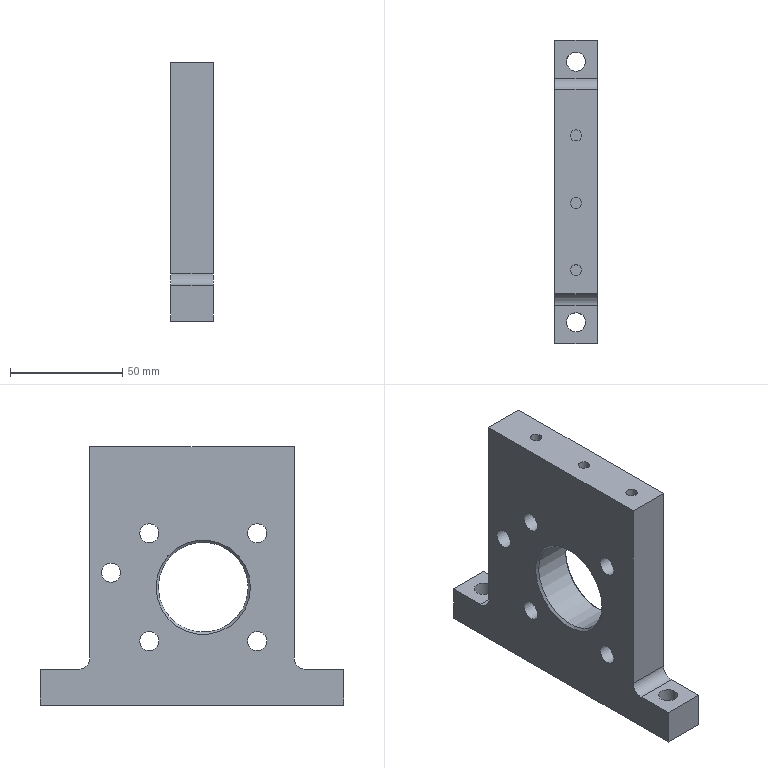CAM job | NX | 3+2 milling, drilling | part box 19 x 135 x 115 mm | stock box 25 x 140 x 120 mm
Tools:
number,name,description,diameter,corner_radius,flute_length,length,flutes
8,D8,平底铣刀-粗,8.0,0.0,30.0,75.0,2
9,D10,平底铣刀-粗,10.0,0.0,35.0,75.0,2
10,D10-J,平底铣刀-精,10.0,0.0,35.0,75.0,2
1,D80R0.8飞刀,圆鼻刀-粗,80.0,0.8,50.0,75.0,2
1,D80R0.8飞刀-J,圆鼻刀-精,80.0,0.8,50.0,75.0,2
2,D6倒角刀,倒角刀,6.0,0.0,3.0,25.0,2
17,ZT8.5,钻头,8.5,0.0,35.0,50.0,2
Operations:
program,operation,operation_type,tool,method,geometry_group,spindle_rpm,surface_speed,feed_per_tooth,feed_cut,feed_plunge,cut_length_mm,path_length_mm,cut_time_min,machine_time_min
B,底壁铣飞面开粗_COPY,VolumeBased25DMillingOperation,D80R0.8飞刀,分层开粗-切深K-步距G,W-B,5000.0,1256.637,0.3,3000.0,100.0,5255.097,5923.505,1.752,1.819
B,底壁铣飞面精光_COPY,VolumeBased25DMillingOperation,D80R0.8飞刀-J,侧刃精光-切深K-步距G,W-B,5000.0,1256.637,0.1,1000.0,100.0,477.149,513.149,0.4771,0.4807
B,平面去毛刺6X45L_COPY,SurfaceContour,D6倒角刀,爬面_倒角-切深0-步距G,W-B,6500.0,122.519,0.1154,1500.0,100.0,626.646,963.301,0.4178,0.4514
B,底壁铣倒角_COPY_1,VolumeBased25DMillingOperation,D6倒角刀,爬面_倒角-切深0-步距G,W-B,6500.0,122.519,0.1154,1500.0,100.0,128.515,168.915,0.0857,0.0897
A,顶面,FaceMilling,D80R0.8飞刀,侧刃精光-切深K-步距G,W-A,5000.0,1256.637,0.1,1000.0,100.0,756.5,792.5,0.7565,0.7601
A,沉头孔打点-深0.8,Operation,D6倒角刀,NONE,W-A,8000.0,150.796,0.0312,500.0,90.0,10.8,255.927,0.0216,0.0461
A,沉头孔-钻孔0段,Operation,ZT8.5,NONE,W-A,1500.0,40.055,0.0833,250.0,90.0,147.322,528.971,0.5893,0.6275
A,动态开粗D10_COPY,CavityMilling,D10,动态开粗-切深K-步距K,W-A,8000.0,251.32,0.25,4000.0,100.0,14664.081,15165.308,3.666,3.716
A,铣孔开粗D8_1,CylinderMilling,D8,NONE,W-A,8000.0,201.062,0.075,1200.0,100.0,1777.188,2185.586,1.481,1.522
A,铣孔精光D8_1,CylinderMilling,D8,精光步距切深关,W-A,8000.0,201.062,0.0312,500.0,100.0,316.687,725.085,0.6334,0.6742
A,仅选体,SurfaceContour,D6倒角刀,METHOD,W-A,8000.0,150.796,0.1875,3000.0,100.0,738.156,1147.526,0.2461,0.287
A,铣倒角_1,PlanarMilling,D6倒角刀,NONE,W-A,8000.0,150.796,0.05,800.0,100.0,264.087,609.639,0.3301,0.3647
A,底壁铣倒角_COPY,VolumeBased25DMillingOperation,D6倒角刀,爬面_倒角-切深0-步距G,W-A,6500.0,122.519,0.1154,1500.0,100.0,128.515,168.915,0.0857,0.0897
A,底壁铣精光侧面-中_COPY,VolumeBased25DMillingOperation,D10-J,侧刃精光-切深K-步距G,W-A,8000.0,251.32,0.0625,1000.0,100.0,205.855,261.859,0.2059,0.2115
A,外形半精_2,VolumeBased25DMillingOperation,D10-J,METHOD,W-A,8000.0,251.327,0.0625,1000.0,100.0,532.082,610.082,0.5321,0.5399